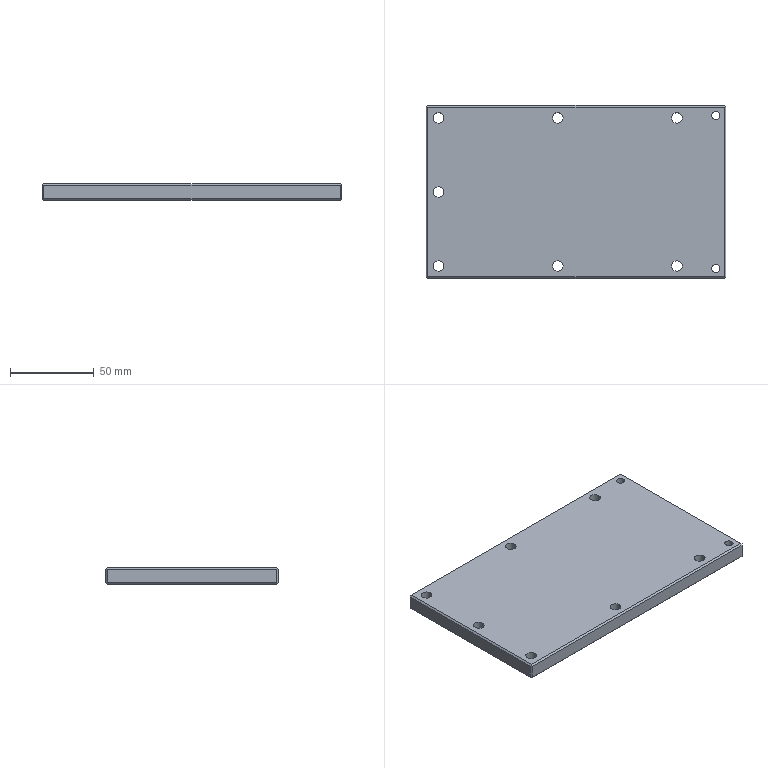Part | Creo | features DATUM PLANE 3, CHAMFER 1, COORDINATE SYSTEM 1, CURVE 1, PROTRUSION 1 | 1 solid | 36 faces | box 179.25 x 103.5 x 10 mm | volume 182337 mm3 | plane 18 | cylinder 18 | commonest cylinder face diameters 6.375 x14 4.875 x4
STEP:
#1=CARTESIAN_POINT('',(0.,0.,0.));
#2=DIRECTION('',(0.,0.,1.));
#3=DIRECTION('',(1.,0.,0.));
#4=AXIS2_PLACEMENT_3D('',#1,#2,#3);
#5=CARTESIAN_POINT('',(-88.63,50.75,0.));
#6=VERTEX_POINT('',#5);
#7=CARTESIAN_POINT('',(88.62,50.75,0.));
#8=VERTEX_POINT('',#7);
#9=CARTESIAN_POINT('',(-88.63,50.75,0.));
#10=DIRECTION('',(1.,0.,0.));
#11=VECTOR('',#10,177.25);
#12=LINE('',#9,#11);
#13=EDGE_CURVE('',#6,#8,#12,.T.);
#14=ORIENTED_EDGE('',*,*,#13,.F.);
#15=CARTESIAN_POINT('',(-88.63,-50.75,0.));
#16=VERTEX_POINT('',#15);
#17=CARTESIAN_POINT('',(-88.63,-50.75,0.));
#18=DIRECTION('',(0.,1.,0.));
#19=VECTOR('',#18,101.5);
#20=LINE('',#17,#19);
#21=EDGE_CURVE('',#16,#6,#20,.T.);
#22=ORIENTED_EDGE('',*,*,#21,.F.);
#23=CARTESIAN_POINT('',(88.62,-50.75,0.));
#24=VERTEX_POINT('',#23);
#25=CARTESIAN_POINT('',(88.62,-50.75,0.));
#26=DIRECTION('',(-1.,0.,0.));
#27=VECTOR('',#26,177.25);
#28=LINE('',#25,#27);
#29=EDGE_CURVE('',#24,#16,#28,.T.);
#30=ORIENTED_EDGE('',*,*,#29,.F.);
#31=CARTESIAN_POINT('',(88.62,50.75,0.));
#32=DIRECTION('',(0.,-1.,0.));
#33=VECTOR('',#32,101.5);
#34=LINE('',#31,#33);
#35=EDGE_CURVE('',#8,#24,#34,.T.);
#36=ORIENTED_EDGE('',*,*,#35,.F.);
#37=EDGE_LOOP('',(#14,#22,#30,#36));
#38=FACE_OUTER_BOUND('',#37,.F.);
#39=CARTESIAN_POINT('',(-78.942,-44.25,0.));
#40=VERTEX_POINT('',#39);
#41=CARTESIAN_POINT('',(-85.317,-44.25,0.));
#42=VERTEX_POINT('',#41);
#43=CARTESIAN_POINT('',(-82.13,-44.25,0.));
#44=DIRECTION('',(0.,0.,-1.));
#45=DIRECTION('',(1.,0.,0.));
#46=AXIS2_PLACEMENT_3D('',#43,#44,#45);
#47=CIRCLE('',#46,3.188);
#48=EDGE_CURVE('',#40,#42,#47,.T.);
#49=ORIENTED_EDGE('',*,*,#48,.T.);
#50=CARTESIAN_POINT('',(-82.13,-44.25,0.));
#51=DIRECTION('',(0.,0.,-1.));
#52=DIRECTION('',(-1.,0.,0.));
#53=AXIS2_PLACEMENT_3D('',#50,#51,#52);
#54=CIRCLE('',#53,3.188);
#55=EDGE_CURVE('',#42,#40,#54,.T.);
#56=ORIENTED_EDGE('',*,*,#55,.T.);
#57=EDGE_LOOP('',(#49,#56));
#58=FACE_BOUND('',#57,.F.);
#59=CARTESIAN_POINT('',(63.557,44.25,0.));
#60=VERTEX_POINT('',#59);
#61=CARTESIAN_POINT('',(57.182,44.25,0.));
#62=VERTEX_POINT('',#61);
#63=CARTESIAN_POINT('',(60.37,44.25,0.));
#64=DIRECTION('',(0.,0.,-1.));
#65=DIRECTION('',(1.,0.,0.));
#66=AXIS2_PLACEMENT_3D('',#63,#64,#65);
#67=CIRCLE('',#66,3.188);
#68=EDGE_CURVE('',#60,#62,#67,.T.);
#69=ORIENTED_EDGE('',*,*,#68,.T.);
#70=CARTESIAN_POINT('',(60.37,44.25,0.));
#71=DIRECTION('',(0.,0.,-1.));
#72=DIRECTION('',(-1.,0.,0.));
#73=AXIS2_PLACEMENT_3D('',#70,#71,#72);
#74=CIRCLE('',#73,3.188);
#75=EDGE_CURVE('',#62,#60,#74,.T.);
#76=ORIENTED_EDGE('',*,*,#75,.T.);
#77=EDGE_LOOP('',(#69,#76));
#78=FACE_BOUND('',#77,.F.);
#79=CARTESIAN_POINT('',(63.557,-44.25,0.));
#80=VERTEX_POINT('',#79);
#81=CARTESIAN_POINT('',(57.182,-44.25,0.));
#82=VERTEX_POINT('',#81);
#83=CARTESIAN_POINT('',(60.37,-44.25,0.));
#84=DIRECTION('',(0.,0.,-1.));
#85=DIRECTION('',(1.,0.,0.));
#86=AXIS2_PLACEMENT_3D('',#83,#84,#85);
#87=CIRCLE('',#86,3.188);
#88=EDGE_CURVE('',#80,#82,#87,.T.);
#89=ORIENTED_EDGE('',*,*,#88,.T.);
#90=CARTESIAN_POINT('',(60.37,-44.25,0.));
#91=DIRECTION('',(0.,0.,-1.));
#92=DIRECTION('',(-1.,0.,0.));
#93=AXIS2_PLACEMENT_3D('',#90,#91,#92);
#94=CIRCLE('',#93,3.188);
#95=EDGE_CURVE('',#82,#80,#94,.T.);
#96=ORIENTED_EDGE('',*,*,#95,.T.);
#97=EDGE_LOOP('',(#89,#96));
#98=FACE_BOUND('',#97,.F.);
#99=CARTESIAN_POINT('',(-7.692,44.25,0.));
#100=VERTEX_POINT('',#99);
#101=CARTESIAN_POINT('',(-14.068,44.25,0.));
#102=VERTEX_POINT('',#101);
#103=CARTESIAN_POINT('',(-10.88,44.25,0.));
#104=DIRECTION('',(0.,0.,-1.));
#105=DIRECTION('',(1.,0.,0.));
#106=AXIS2_PLACEMENT_3D('',#103,#104,#105);
#107=CIRCLE('',#106,3.188);
#108=EDGE_CURVE('',#100,#102,#107,.T.);
#109=ORIENTED_EDGE('',*,*,#108,.T.);
#110=CARTESIAN_POINT('',(-10.88,44.25,0.));
#111=DIRECTION('',(0.,0.,-1.));
#112=DIRECTION('',(-1.,0.,0.));
#113=AXIS2_PLACEMENT_3D('',#110,#111,#112);
#114=CIRCLE('',#113,3.188);
#115=EDGE_CURVE('',#102,#100,#114,.T.);
#116=ORIENTED_EDGE('',*,*,#115,.T.);
#117=EDGE_LOOP('',(#109,#116));
#118=FACE_BOUND('',#117,.F.);
#119=CARTESIAN_POINT('',(-7.692,-44.25,0.));
#120=VERTEX_POINT('',#119);
#121=CARTESIAN_POINT('',(-14.068,-44.25,0.));
#122=VERTEX_POINT('',#121);
#123=CARTESIAN_POINT('',(-10.88,-44.25,0.));
#124=DIRECTION('',(0.,0.,-1.));
#125=DIRECTION('',(1.,0.,0.));
#126=AXIS2_PLACEMENT_3D('',#123,#124,#125);
#127=CIRCLE('',#126,3.188);
#128=EDGE_CURVE('',#120,#122,#127,.T.);
#129=ORIENTED_EDGE('',*,*,#128,.T.);
#130=CARTESIAN_POINT('',(-10.88,-44.25,0.));
#131=DIRECTION('',(0.,0.,-1.));
#132=DIRECTION('',(-1.,0.,0.));
#133=AXIS2_PLACEMENT_3D('',#130,#131,#132);
#134=CIRCLE('',#133,3.188);
#135=EDGE_CURVE('',#122,#120,#134,.T.);
#136=ORIENTED_EDGE('',*,*,#135,.T.);
#137=EDGE_LOOP('',(#129,#136));
#138=FACE_BOUND('',#137,.F.);
#139=CARTESIAN_POINT('',(-78.942,0.,0.));
#140=VERTEX_POINT('',#139);
#141=CARTESIAN_POINT('',(-85.317,0.,0.));
#142=VERTEX_POINT('',#141);
#143=CARTESIAN_POINT('',(-82.13,0.,0.));
#144=DIRECTION('',(0.,0.,-1.));
#145=DIRECTION('',(1.,0.,0.));
#146=AXIS2_PLACEMENT_3D('',#143,#144,#145);
#147=CIRCLE('',#146,3.188);
#148=EDGE_CURVE('',#140,#142,#147,.T.);
#149=ORIENTED_EDGE('',*,*,#148,.T.);
#150=CARTESIAN_POINT('',(-82.13,0.,0.));
#151=DIRECTION('',(0.,0.,-1.));
#152=DIRECTION('',(-1.,0.,0.));
#153=AXIS2_PLACEMENT_3D('',#150,#151,#152);
#154=CIRCLE('',#153,3.188);
#155=EDGE_CURVE('',#142,#140,#154,.T.);
#156=ORIENTED_EDGE('',*,*,#155,.T.);
#157=EDGE_LOOP('',(#149,#156));
#158=FACE_BOUND('',#157,.F.);
#159=CARTESIAN_POINT('',(86.058,45.75,0.));
#160=VERTEX_POINT('',#159);
#161=CARTESIAN_POINT('',(81.183,45.75,0.));
#162=VERTEX_POINT('',#161);
#163=CARTESIAN_POINT('',(83.62,45.75,0.));
#164=DIRECTION('',(0.,0.,-1.));
#165=DIRECTION('',(1.,0.,0.));
#166=AXIS2_PLACEMENT_3D('',#163,#164,#165);
#167=CIRCLE('',#166,2.438);
#168=EDGE_CURVE('',#160,#162,#167,.T.);
#169=ORIENTED_EDGE('',*,*,#168,.T.);
#170=CARTESIAN_POINT('',(83.62,45.75,0.));
#171=DIRECTION('',(0.,0.,-1.));
#172=DIRECTION('',(-1.,0.,0.));
#173=AXIS2_PLACEMENT_3D('',#170,#171,#172);
#174=CIRCLE('',#173,2.438);
#175=EDGE_CURVE('',#162,#160,#174,.T.);
#176=ORIENTED_EDGE('',*,*,#175,.T.);
#177=EDGE_LOOP('',(#169,#176));
#178=FACE_BOUND('',#177,.F.);
#179=CARTESIAN_POINT('',(86.058,-45.75,0.));
#180=VERTEX_POINT('',#179);
#181=CARTESIAN_POINT('',(81.183,-45.75,0.));
#182=VERTEX_POINT('',#181);
#183=CARTESIAN_POINT('',(83.62,-45.75,0.));
#184=DIRECTION('',(0.,0.,-1.));
#185=DIRECTION('',(1.,0.,0.));
#186=AXIS2_PLACEMENT_3D('',#183,#184,#185);
#187=CIRCLE('',#186,2.438);
#188=EDGE_CURVE('',#180,#182,#187,.T.);
#189=ORIENTED_EDGE('',*,*,#188,.T.);
#190=CARTESIAN_POINT('',(83.62,-45.75,0.));
#191=DIRECTION('',(0.,0.,-1.));
#192=DIRECTION('',(-1.,0.,0.));
#193=AXIS2_PLACEMENT_3D('',#190,#191,#192);
#194=CIRCLE('',#193,2.438);
#195=EDGE_CURVE('',#182,#180,#194,.T.);
#196=ORIENTED_EDGE('',*,*,#195,.T.);
#197=EDGE_LOOP('',(#189,#196));
#198=FACE_BOUND('',#197,.F.);
#199=CARTESIAN_POINT('',(-78.942,44.25,0.));
#200=VERTEX_POINT('',#199);
#201=CARTESIAN_POINT('',(-85.317,44.25,0.));
#202=VERTEX_POINT('',#201);
#203=CARTESIAN_POINT('',(-82.13,44.25,0.));
#204=DIRECTION('',(0.,0.,-1.));
#205=DIRECTION('',(1.,0.,0.));
#206=AXIS2_PLACEMENT_3D('',#203,#204,#205);
#207=CIRCLE('',#206,3.188);
#208=EDGE_CURVE('',#200,#202,#207,.T.);
#209=ORIENTED_EDGE('',*,*,#208,.T.);
#210=CARTESIAN_POINT('',(-82.13,44.25,0.));
#211=DIRECTION('',(0.,0.,-1.));
#212=DIRECTION('',(-1.,0.,0.));
#213=AXIS2_PLACEMENT_3D('',#210,#211,#212);
#214=CIRCLE('',#213,3.188);
#215=EDGE_CURVE('',#202,#200,#214,.T.);
#216=ORIENTED_EDGE('',*,*,#215,.T.);
#217=EDGE_LOOP('',(#209,#216));
#218=FACE_BOUND('',#217,.F.);
#219=CARTESIAN_POINT('',(0.,0.,0.));
#220=DIRECTION('',(0.,0.,1.));
#221=DIRECTION('',(1.,0.,0.));
#222=AXIS2_PLACEMENT_3D('',#219,#220,#221);
#223=PLANE('',#222);
#224=ADVANCED_FACE('',(#38,#58,#78,#98,#118,#138,#158,#178,#198,#218),#223,.F.);
#225=ORIENTED_EDGE('',*,*,#208,.F.);
#226=CARTESIAN_POINT('',(-78.942,44.25,10.));
#227=VERTEX_POINT('',#226);
#228=CARTESIAN_POINT('',(-78.942,44.25,0.));
#229=DIRECTION('',(0.,0.,1.));
#230=VECTOR('',#229,10.);
#231=LINE('',#228,#230);
#232=EDGE_CURVE('',#200,#227,#231,.T.);
#233=ORIENTED_EDGE('',*,*,#232,.T.);
#234=CARTESIAN_POINT('',(-85.317,44.25,10.));
#235=VERTEX_POINT('',#234);
#236=CARTESIAN_POINT('',(-82.13,44.25,10.));
#237=DIRECTION('',(0.,0.,-1.));
#238=DIRECTION('',(1.,0.,0.));
#239=AXIS2_PLACEMENT_3D('',#236,#237,#238);
#240=CIRCLE('',#239,3.188);
#241=EDGE_CURVE('',#227,#235,#240,.T.);
#242=ORIENTED_EDGE('',*,*,#241,.T.);
#243=CARTESIAN_POINT('',(-85.317,44.25,0.));
#244=DIRECTION('',(0.,0.,1.));
#245=VECTOR('',#244,10.);
#246=LINE('',#243,#245);
#247=EDGE_CURVE('',#202,#235,#246,.T.);
#248=ORIENTED_EDGE('',*,*,#247,.F.);
#249=EDGE_LOOP('',(#225,#233,#242,#248));
#250=FACE_OUTER_BOUND('',#249,.F.);
#251=CARTESIAN_POINT('',(-82.13,44.25,0.));
#252=DIRECTION('',(0.,0.,1.));
#253=DIRECTION('',(1.,0.,0.));
#254=AXIS2_PLACEMENT_3D('',#251,#252,#253);
#255=CYLINDRICAL_SURFACE('',#254,3.188);
#256=ADVANCED_FACE('',(#250),#255,.F.);
#257=ORIENTED_EDGE('',*,*,#215,.F.);
#258=ORIENTED_EDGE('',*,*,#247,.T.);
#259=CARTESIAN_POINT('',(-82.13,44.25,10.));
#260=DIRECTION('',(0.,0.,-1.));
#261=DIRECTION('',(-1.,0.,0.));
#262=AXIS2_PLACEMENT_3D('',#259,#260,#261);
#263=CIRCLE('',#262,3.188);
#264=EDGE_CURVE('',#235,#227,#263,.T.);
#265=ORIENTED_EDGE('',*,*,#264,.T.);
#266=ORIENTED_EDGE('',*,*,#232,.F.);
#267=EDGE_LOOP('',(#257,#258,#265,#266));
#268=FACE_OUTER_BOUND('',#267,.F.);
#269=CARTESIAN_POINT('',(-82.13,44.25,0.));
#270=DIRECTION('',(0.,0.,1.));
#271=DIRECTION('',(1.,0.,0.));
#272=AXIS2_PLACEMENT_3D('',#269,#270,#271);
#273=CYLINDRICAL_SURFACE('',#272,3.188);
#274=ADVANCED_FACE('',(#268),#273,.F.);
#275=CARTESIAN_POINT('',(88.62,-50.75,10.));
#276=VERTEX_POINT('',#275);
#277=CARTESIAN_POINT('',(88.62,50.75,10.));
#278=VERTEX_POINT('',#277);
#279=CARTESIAN_POINT('',(88.62,-50.75,10.));
#280=DIRECTION('',(0.,1.,0.));
#281=VECTOR('',#280,101.5);
#282=LINE('',#279,#281);
#283=EDGE_CURVE('',#276,#278,#282,.T.);
#284=ORIENTED_EDGE('',*,*,#283,.F.);
#285=CARTESIAN_POINT('',(-88.63,-50.75,10.));
#286=VERTEX_POINT('',#285);
#287=CARTESIAN_POINT('',(-88.63,-50.75,10.));
#288=DIRECTION('',(1.,0.,0.));
#289=VECTOR('',#288,177.25);
#290=LINE('',#287,#289);
#291=EDGE_CURVE('',#286,#276,#290,.T.);
#292=ORIENTED_EDGE('',*,*,#291,.F.);
#293=CARTESIAN_POINT('',(-88.63,50.75,10.));
#294=VERTEX_POINT('',#293);
#295=CARTESIAN_POINT('',(-88.63,50.75,10.));
#296=DIRECTION('',(0.,-1.,0.));
#297=VECTOR('',#296,101.5);
#298=LINE('',#295,#297);
#299=EDGE_CURVE('',#294,#286,#298,.T.);
#300=ORIENTED_EDGE('',*,*,#299,.F.);
#301=CARTESIAN_POINT('',(88.62,50.75,10.));
#302=DIRECTION('',(-1.,0.,0.));
#303=VECTOR('',#302,177.25);
#304=LINE('',#301,#303);
#305=EDGE_CURVE('',#278,#294,#304,.T.);
#306=ORIENTED_EDGE('',*,*,#305,.F.);
#307=EDGE_LOOP('',(#284,#292,#300,#306));
#308=FACE_OUTER_BOUND('',#307,.F.);
#309=CARTESIAN_POINT('',(-78.942,-44.25,10.));
#310=VERTEX_POINT('',#309);
#311=CARTESIAN_POINT('',(-85.317,-44.25,10.));
#312=VERTEX_POINT('',#311);
#313=CARTESIAN_POINT('',(-82.13,-44.25,10.));
#314=DIRECTION('',(0.,0.,-1.));
#315=DIRECTION('',(1.,0.,0.));
#316=AXIS2_PLACEMENT_3D('',#313,#314,#315);
#317=CIRCLE('',#316,3.188);
#318=EDGE_CURVE('',#310,#312,#317,.T.);
#319=ORIENTED_EDGE('',*,*,#318,.F.);
#320=CARTESIAN_POINT('',(-82.13,-44.25,10.));
#321=DIRECTION('',(0.,0.,-1.));
#322=DIRECTION('',(-1.,0.,0.));
#323=AXIS2_PLACEMENT_3D('',#320,#321,#322);
#324=CIRCLE('',#323,3.188);
#325=EDGE_CURVE('',#312,#310,#324,.T.);
#326=ORIENTED_EDGE('',*,*,#325,.F.);
#327=EDGE_LOOP('',(#319,#326));
#328=FACE_BOUND('',#327,.F.);
#329=CARTESIAN_POINT('',(63.557,44.25,10.));
#330=VERTEX_POINT('',#329);
#331=CARTESIAN_POINT('',(57.182,44.25,10.));
#332=VERTEX_POINT('',#331);
#333=CARTESIAN_POINT('',(60.37,44.25,10.));
#334=DIRECTION('',(0.,0.,-1.));
#335=DIRECTION('',(1.,0.,0.));
#336=AXIS2_PLACEMENT_3D('',#333,#334,#335);
#337=CIRCLE('',#336,3.188);
#338=EDGE_CURVE('',#330,#332,#337,.T.);
#339=ORIENTED_EDGE('',*,*,#338,.F.);
#340=CARTESIAN_POINT('',(60.37,44.25,10.));
#341=DIRECTION('',(0.,0.,-1.));
#342=DIRECTION('',(-1.,0.,0.));
#343=AXIS2_PLACEMENT_3D('',#340,#341,#342);
#344=CIRCLE('',#343,3.188);
#345=EDGE_CURVE('',#332,#330,#344,.T.);
#346=ORIENTED_EDGE('',*,*,#345,.F.);
#347=EDGE_LOOP('',(#339,#346));
#348=FACE_BOUND('',#347,.F.);
#349=CARTESIAN_POINT('',(63.557,-44.25,10.));
#350=VERTEX_POINT('',#349);
#351=CARTESIAN_POINT('',(57.182,-44.25,10.));
#352=VERTEX_POINT('',#351);
#353=CARTESIAN_POINT('',(60.37,-44.25,10.));
#354=DIRECTION('',(0.,0.,-1.));
#355=DIRECTION('',(1.,0.,0.));
#356=AXIS2_PLACEMENT_3D('',#353,#354,#355);
#357=CIRCLE('',#356,3.188);
#358=EDGE_CURVE('',#350,#352,#357,.T.);
#359=ORIENTED_EDGE('',*,*,#358,.F.);
#360=CARTESIAN_POINT('',(60.37,-44.25,10.));
#361=DIRECTION('',(0.,0.,-1.));
#362=DIRECTION('',(-1.,0.,0.));
#363=AXIS2_PLACEMENT_3D('',#360,#361,#362);
#364=CIRCLE('',#363,3.188);
#365=EDGE_CURVE('',#352,#350,#364,.T.);
#366=ORIENTED_EDGE('',*,*,#365,.F.);
#367=EDGE_LOOP('',(#359,#366));
#368=FACE_BOUND('',#367,.F.);
#369=CARTESIAN_POINT('',(-7.692,44.25,10.));
#370=VERTEX_POINT('',#369);
#371=CARTESIAN_POINT('',(-14.068,44.25,10.));
#372=VERTEX_POINT('',#371);
#373=CARTESIAN_POINT('',(-10.88,44.25,10.));
#374=DIRECTION('',(0.,0.,-1.));
#375=DIRECTION('',(1.,0.,0.));
#376=AXIS2_PLACEMENT_3D('',#373,#374,#375);
#377=CIRCLE('',#376,3.188);
#378=EDGE_CURVE('',#370,#372,#377,.T.);
#379=ORIENTED_EDGE('',*,*,#378,.F.);
#380=CARTESIAN_POINT('',(-10.88,44.25,10.));
#381=DIRECTION('',(0.,0.,-1.));
#382=DIRECTION('',(-1.,0.,0.));
#383=AXIS2_PLACEMENT_3D('',#380,#381,#382);
#384=CIRCLE('',#383,3.188);
#385=EDGE_CURVE('',#372,#370,#384,.T.);
#386=ORIENTED_EDGE('',*,*,#385,.F.);
#387=EDGE_LOOP('',(#379,#386));
#388=FACE_BOUND('',#387,.F.);
#389=CARTESIAN_POINT('',(-7.692,-44.25,10.));
#390=VERTEX_POINT('',#389);
#391=CARTESIAN_POINT('',(-14.068,-44.25,10.));
#392=VERTEX_POINT('',#391);
#393=CARTESIAN_POINT('',(-10.88,-44.25,10.));
#394=DIRECTION('',(0.,0.,-1.));
#395=DIRECTION('',(1.,0.,0.));
#396=AXIS2_PLACEMENT_3D('',#393,#394,#395);
#397=CIRCLE('',#396,3.188);
#398=EDGE_CURVE('',#390,#392,#397,.T.);
#399=ORIENTED_EDGE('',*,*,#398,.F.);
#400=CARTESIAN_POINT('',(-10.88,-44.25,10.));
#401=DIRECTION('',(0.,0.,-1.));
#402=DIRECTION('',(-1.,0.,0.));
#403=AXIS2_PLACEMENT_3D('',#400,#401,#402);
#404=CIRCLE('',#403,3.188);
#405=EDGE_CURVE('',#392,#390,#404,.T.);
#406=ORIENTED_EDGE('',*,*,#405,.F.);
#407=EDGE_LOOP('',(#399,#406));
#408=FACE_BOUND('',#407,.F.);
#409=CARTESIAN_POINT('',(-78.942,0.,10.));
#410=VERTEX_POINT('',#409);
#411=CARTESIAN_POINT('',(-85.317,0.,10.));
#412=VERTEX_POINT('',#411);
#413=CARTESIAN_POINT('',(-82.13,0.,10.));
#414=DIRECTION('',(0.,0.,-1.));
#415=DIRECTION('',(1.,0.,0.));
#416=AXIS2_PLACEMENT_3D('',#413,#414,#415);
#417=CIRCLE('',#416,3.188);
#418=EDGE_CURVE('',#410,#412,#417,.T.);
#419=ORIENTED_EDGE('',*,*,#418,.F.);
#420=CARTESIAN_POINT('',(-82.13,0.,10.));
#421=DIRECTION('',(0.,0.,-1.));
#422=DIRECTION('',(-1.,0.,0.));
#423=AXIS2_PLACEMENT_3D('',#420,#421,#422);
#424=CIRCLE('',#423,3.188);
#425=EDGE_CURVE('',#412,#410,#424,.T.);
#426=ORIENTED_EDGE('',*,*,#425,.F.);
#427=EDGE_LOOP('',(#419,#426));
#428=FACE_BOUND('',#427,.F.);
#429=CARTESIAN_POINT('',(86.058,45.75,10.));
#430=VERTEX_POINT('',#429);
#431=CARTESIAN_POINT('',(81.183,45.75,10.));
#432=VERTEX_POINT('',#431);
#433=CARTESIAN_POINT('',(83.62,45.75,10.));
#434=DIRECTION('',(0.,0.,-1.));
#435=DIRECTION('',(1.,0.,0.));
#436=AXIS2_PLACEMENT_3D('',#433,#434,#435);
#437=CIRCLE('',#436,2.438);
#438=EDGE_CURVE('',#430,#432,#437,.T.);
#439=ORIENTED_EDGE('',*,*,#438,.F.);
#440=CARTESIAN_POINT('',(83.62,45.75,10.));
#441=DIRECTION('',(0.,0.,-1.));
#442=DIRECTION('',(-1.,0.,0.));
#443=AXIS2_PLACEMENT_3D('',#440,#441,#442);
#444=CIRCLE('',#443,2.438);
#445=EDGE_CURVE('',#432,#430,#444,.T.);
#446=ORIENTED_EDGE('',*,*,#445,.F.);
#447=EDGE_LOOP('',(#439,#446));
#448=FACE_BOUND('',#447,.F.);
#449=CARTESIAN_POINT('',(86.058,-45.75,10.));
#450=VERTEX_POINT('',#449);
#451=CARTESIAN_POINT('',(81.183,-45.75,10.));
#452=VERTEX_POINT('',#451);
#453=CARTESIAN_POINT('',(83.62,-45.75,10.));
#454=DIRECTION('',(0.,0.,-1.));
#455=DIRECTION('',(1.,0.,0.));
#456=AXIS2_PLACEMENT_3D('',#453,#454,#455);
#457=CIRCLE('',#456,2.438);
#458=EDGE_CURVE('',#450,#452,#457,.T.);
#459=ORIENTED_EDGE('',*,*,#458,.F.);
#460=CARTESIAN_POINT('',(83.62,-45.75,10.));
#461=DIRECTION('',(0.,0.,-1.));
#462=DIRECTION('',(-1.,0.,0.));
#463=AXIS2_PLACEMENT_3D('',#460,#461,#462);
#464=CIRCLE('',#463,2.438);
#465=EDGE_CURVE('',#452,#450,#464,.T.);
#466=ORIENTED_EDGE('',*,*,#465,.F.);
#467=EDGE_LOOP('',(#459,#466));
#468=FACE_BOUND('',#467,.F.);
#469=ORIENTED_EDGE('',*,*,#241,.F.);
#470=ORIENTED_EDGE('',*,*,#264,.F.);
#471=EDGE_LOOP('',(#469,#470));
#472=FACE_BOUND('',#471,.F.);
#473=CARTESIAN_POINT('',(0.,0.,10.));
#474=DIRECTION('',(0.,0.,1.));
#475=DIRECTION('',(1.,0.,0.));
#476=AXIS2_PLACEMENT_3D('',#473,#474,#475);
#477=PLANE('',#476);
#478=ADVANCED_FACE('',(#308,#328,#348,#368,#388,#408,#428,#448,#468,#472),#477,.T.);
#479=ORIENTED_EDGE('',*,*,#48,.F.);
#480=CARTESIAN_POINT('',(-78.942,-44.25,0.));
#481=DIRECTION('',(0.,0.,1.));
#482=VECTOR('',#481,10.);
#483=LINE('',#480,#482);
#484=EDGE_CURVE('',#40,#310,#483,.T.);
#485=ORIENTED_EDGE('',*,*,#484,.T.);
#486=ORIENTED_EDGE('',*,*,#318,.T.);
#487=CARTESIAN_POINT('',(-85.317,-44.25,0.));
#488=DIRECTION('',(0.,0.,1.));
#489=VECTOR('',#488,10.);
#490=LINE('',#487,#489);
#491=EDGE_CURVE('',#42,#312,#490,.T.);
#492=ORIENTED_EDGE('',*,*,#491,.F.);
#493=EDGE_LOOP('',(#479,#485,#486,#492));
#494=FACE_OUTER_BOUND('',#493,.F.);
#495=CARTESIAN_POINT('',(-82.13,-44.25,0.));
#496=DIRECTION('',(0.,0.,1.));
#497=DIRECTION('',(1.,0.,0.));
#498=AXIS2_PLACEMENT_3D('',#495,#496,#497);
#499=CYLINDRICAL_SURFACE('',#498,3.188);
#500=ADVANCED_FACE('',(#494),#499,.F.);
#501=ORIENTED_EDGE('',*,*,#55,.F.);
#502=ORIENTED_EDGE('',*,*,#491,.T.);
#503=ORIENTED_EDGE('',*,*,#325,.T.);
#504=ORIENTED_EDGE('',*,*,#484,.F.);
#505=EDGE_LOOP('',(#501,#502,#503,#504));
#506=FACE_OUTER_BOUND('',#505,.F.);
#507=CARTESIAN_POINT('',(-82.13,-44.25,0.));
#508=DIRECTION('',(0.,0.,1.));
#509=DIRECTION('',(1.,0.,0.));
#510=AXIS2_PLACEMENT_3D('',#507,#508,#509);
#511=CYLINDRICAL_SURFACE('',#510,3.188);
#512=ADVANCED_FACE('',(#506),#511,.F.);
#513=ORIENTED_EDGE('',*,*,#68,.F.);
#514=CARTESIAN_POINT('',(63.557,44.25,0.));
#515=DIRECTION('',(0.,0.,1.));
#516=VECTOR('',#515,10.);
#517=LINE('',#514,#516);
#518=EDGE_CURVE('',#60,#330,#517,.T.);
#519=ORIENTED_EDGE('',*,*,#518,.T.);
#520=ORIENTED_EDGE('',*,*,#338,.T.);
#521=CARTESIAN_POINT('',(57.182,44.25,0.));
#522=DIRECTION('',(0.,0.,1.));
#523=VECTOR('',#522,10.);
#524=LINE('',#521,#523);
#525=EDGE_CURVE('',#62,#332,#524,.T.);
#526=ORIENTED_EDGE('',*,*,#525,.F.);
#527=EDGE_LOOP('',(#513,#519,#520,#526));
#528=FACE_OUTER_BOUND('',#527,.F.);
#529=CARTESIAN_POINT('',(60.37,44.25,0.));
#530=DIRECTION('',(0.,0.,1.));
#531=DIRECTION('',(1.,0.,0.));
#532=AXIS2_PLACEMENT_3D('',#529,#530,#531);
#533=CYLINDRICAL_SURFACE('',#532,3.188);
#534=ADVANCED_FACE('',(#528),#533,.F.);
#535=ORIENTED_EDGE('',*,*,#75,.F.);
#536=ORIENTED_EDGE('',*,*,#525,.T.);
#537=ORIENTED_EDGE('',*,*,#345,.T.);
#538=ORIENTED_EDGE('',*,*,#518,.F.);
#539=EDGE_LOOP('',(#535,#536,#537,#538));
#540=FACE_OUTER_BOUND('',#539,.F.);
#541=CARTESIAN_POINT('',(60.37,44.25,0.));
#542=DIRECTION('',(0.,0.,1.));
#543=DIRECTION('',(1.,0.,0.));
#544=AXIS2_PLACEMENT_3D('',#541,#542,#543);
#545=CYLINDRICAL_SURFACE('',#544,3.188);
#546=ADVANCED_FACE('',(#540),#545,.F.);
#547=ORIENTED_EDGE('',*,*,#88,.F.);
#548=CARTESIAN_POINT('',(63.557,-44.25,0.));
#549=DIRECTION('',(0.,0.,1.));
#550=VECTOR('',#549,10.);
#551=LINE('',#548,#550);
#552=EDGE_CURVE('',#80,#350,#551,.T.);
#553=ORIENTED_EDGE('',*,*,#552,.T.);
#554=ORIENTED_EDGE('',*,*,#358,.T.);
#555=CARTESIAN_POINT('',(57.182,-44.25,0.));
#556=DIRECTION('',(0.,0.,1.));
#557=VECTOR('',#556,10.);
#558=LINE('',#555,#557);
#559=EDGE_CURVE('',#82,#352,#558,.T.);
#560=ORIENTED_EDGE('',*,*,#559,.F.);
#561=EDGE_LOOP('',(#547,#553,#554,#560));
#562=FACE_OUTER_BOUND('',#561,.F.);
#563=CARTESIAN_POINT('',(60.37,-44.25,0.));
#564=DIRECTION('',(0.,0.,1.));
#565=DIRECTION('',(1.,0.,0.));
#566=AXIS2_PLACEMENT_3D('',#563,#564,#565);
#567=CYLINDRICAL_SURFACE('',#566,3.188);
#568=ADVANCED_FACE('',(#562),#567,.F.);
#569=ORIENTED_EDGE('',*,*,#95,.F.);
#570=ORIENTED_EDGE('',*,*,#559,.T.);
#571=ORIENTED_EDGE('',*,*,#365,.T.);
#572=ORIENTED_EDGE('',*,*,#552,.F.);
#573=EDGE_LOOP('',(#569,#570,#571,#572));
#574=FACE_OUTER_BOUND('',#573,.F.);
#575=CARTESIAN_POINT('',(60.37,-44.25,0.));
#576=DIRECTION('',(0.,0.,1.));
#577=DIRECTION('',(1.,0.,0.));
#578=AXIS2_PLACEMENT_3D('',#575,#576,#577);
#579=CYLINDRICAL_SURFACE('',#578,3.188);
#580=ADVANCED_FACE('',(#574),#579,.F.);
#581=ORIENTED_EDGE('',*,*,#108,.F.);
#582=CARTESIAN_POINT('',(-7.692,44.25,0.));
#583=DIRECTION('',(0.,0.,1.));
#584=VECTOR('',#583,10.);
#585=LINE('',#582,#584);
#586=EDGE_CURVE('',#100,#370,#585,.T.);
#587=ORIENTED_EDGE('',*,*,#586,.T.);
#588=ORIENTED_EDGE('',*,*,#378,.T.);
#589=CARTESIAN_POINT('',(-14.068,44.25,0.));
#590=DIRECTION('',(0.,0.,1.));
#591=VECTOR('',#590,10.);
#592=LINE('',#589,#591);
#593=EDGE_CURVE('',#102,#372,#592,.T.);
#594=ORIENTED_EDGE('',*,*,#593,.F.);
#595=EDGE_LOOP('',(#581,#587,#588,#594));
#596=FACE_OUTER_BOUND('',#595,.F.);
#597=CARTESIAN_POINT('',(-10.88,44.25,0.));
#598=DIRECTION('',(0.,0.,1.));
#599=DIRECTION('',(1.,0.,0.));
#600=AXIS2_PLACEMENT_3D('',#597,#598,#599);
#601=CYLINDRICAL_SURFACE('',#600,3.188);
#602=ADVANCED_FACE('',(#596),#601,.F.);
#603=ORIENTED_EDGE('',*,*,#115,.F.);
#604=ORIENTED_EDGE('',*,*,#593,.T.);
#605=ORIENTED_EDGE('',*,*,#385,.T.);
#606=ORIENTED_EDGE('',*,*,#586,.F.);
#607=EDGE_LOOP('',(#603,#604,#605,#606));
#608=FACE_OUTER_BOUND('',#607,.F.);
#609=CARTESIAN_POINT('',(-10.88,44.25,0.));
#610=DIRECTION('',(0.,0.,1.));
#611=DIRECTION('',(1.,0.,0.));
#612=AXIS2_PLACEMENT_3D('',#609,#610,#611);
#613=CYLINDRICAL_SURFACE('',#612,3.188);
#614=ADVANCED_FACE('',(#608),#613,.F.);
#615=ORIENTED_EDGE('',*,*,#128,.F.);
#616=CARTESIAN_POINT('',(-7.692,-44.25,0.));
#617=DIRECTION('',(0.,0.,1.));
#618=VECTOR('',#617,10.);
#619=LINE('',#616,#618);
#620=EDGE_CURVE('',#120,#390,#619,.T.);
#621=ORIENTED_EDGE('',*,*,#620,.T.);
#622=ORIENTED_EDGE('',*,*,#398,.T.);
#623=CARTESIAN_POINT('',(-14.068,-44.25,0.));
#624=DIRECTION('',(0.,0.,1.));
#625=VECTOR('',#624,10.);
#626=LINE('',#623,#625);
#627=EDGE_CURVE('',#122,#392,#626,.T.);
#628=ORIENTED_EDGE('',*,*,#627,.F.);
#629=EDGE_LOOP('',(#615,#621,#622,#628));
#630=FACE_OUTER_BOUND('',#629,.F.);
#631=CARTESIAN_POINT('',(-10.88,-44.25,0.));
#632=DIRECTION('',(0.,0.,1.));
#633=DIRECTION('',(1.,0.,0.));
#634=AXIS2_PLACEMENT_3D('',#631,#632,#633);
#635=CYLINDRICAL_SURFACE('',#634,3.188);
#636=ADVANCED_FACE('',(#630),#635,.F.);
#637=ORIENTED_EDGE('',*,*,#135,.F.);
#638=ORIENTED_EDGE('',*,*,#627,.T.);
#639=ORIENTED_EDGE('',*,*,#405,.T.);
#640=ORIENTED_EDGE('',*,*,#620,.F.);
#641=EDGE_LOOP('',(#637,#638,#639,#640));
#642=FACE_OUTER_BOUND('',#641,.F.);
#643=CARTESIAN_POINT('',(-10.88,-44.25,0.));
#644=DIRECTION('',(0.,0.,1.));
#645=DIRECTION('',(1.,0.,0.));
#646=AXIS2_PLACEMENT_3D('',#643,#644,#645);
#647=CYLINDRICAL_SURFACE('',#646,3.188);
#648=ADVANCED_FACE('',(#642),#647,.F.);
#649=ORIENTED_EDGE('',*,*,#148,.F.);
#650=CARTESIAN_POINT('',(-78.942,0.,0.));
#651=DIRECTION('',(0.,0.,1.));
#652=VECTOR('',#651,10.);
#653=LINE('',#650,#652);
#654=EDGE_CURVE('',#140,#410,#653,.T.);
#655=ORIENTED_EDGE('',*,*,#654,.T.);
#656=ORIENTED_EDGE('',*,*,#418,.T.);
#657=CARTESIAN_POINT('',(-85.317,0.,0.));
#658=DIRECTION('',(0.,0.,1.));
#659=VECTOR('',#658,10.);
#660=LINE('',#657,#659);
#661=EDGE_CURVE('',#142,#412,#660,.T.);
#662=ORIENTED_EDGE('',*,*,#661,.F.);
#663=EDGE_LOOP('',(#649,#655,#656,#662));
#664=FACE_OUTER_BOUND('',#663,.F.);
#665=CARTESIAN_POINT('',(-82.13,0.,0.));
#666=DIRECTION('',(0.,0.,1.));
#667=DIRECTION('',(1.,0.,0.));
#668=AXIS2_PLACEMENT_3D('',#665,#666,#667);
#669=CYLINDRICAL_SURFACE('',#668,3.188);
#670=ADVANCED_FACE('',(#664),#669,.F.);
#671=ORIENTED_EDGE('',*,*,#155,.F.);
#672=ORIENTED_EDGE('',*,*,#661,.T.);
#673=ORIENTED_EDGE('',*,*,#425,.T.);
#674=ORIENTED_EDGE('',*,*,#654,.F.);
#675=EDGE_LOOP('',(#671,#672,#673,#674));
#676=FACE_OUTER_BOUND('',#675,.F.);
#677=CARTESIAN_POINT('',(-82.13,0.,0.));
#678=DIRECTION('',(0.,0.,1.));
#679=DIRECTION('',(1.,0.,0.));
#680=AXIS2_PLACEMENT_3D('',#677,#678,#679);
#681=CYLINDRICAL_SURFACE('',#680,3.188);
#682=ADVANCED_FACE('',(#676),#681,.F.);
#683=ORIENTED_EDGE('',*,*,#168,.F.);
#684=CARTESIAN_POINT('',(86.058,45.75,0.));
#685=DIRECTION('',(0.,0.,1.));
#686=VECTOR('',#685,10.);
#687=LINE('',#684,#686);
#688=EDGE_CURVE('',#160,#430,#687,.T.);
#689=ORIENTED_EDGE('',*,*,#688,.T.);
#690=ORIENTED_EDGE('',*,*,#438,.T.);
#691=CARTESIAN_POINT('',(81.183,45.75,0.));
#692=DIRECTION('',(0.,0.,1.));
#693=VECTOR('',#692,10.);
#694=LINE('',#691,#693);
#695=EDGE_CURVE('',#162,#432,#694,.T.);
#696=ORIENTED_EDGE('',*,*,#695,.F.);
#697=EDGE_LOOP('',(#683,#689,#690,#696));
#698=FACE_OUTER_BOUND('',#697,.F.);
#699=CARTESIAN_POINT('',(83.62,45.75,0.));
#700=DIRECTION('',(0.,0.,1.));
#701=DIRECTION('',(1.,0.,0.));
#702=AXIS2_PLACEMENT_3D('',#699,#700,#701);
#703=CYLINDRICAL_SURFACE('',#702,2.438);
#704=ADVANCED_FACE('',(#698),#703,.F.);
#705=ORIENTED_EDGE('',*,*,#175,.F.);
#706=ORIENTED_EDGE('',*,*,#695,.T.);
#707=ORIENTED_EDGE('',*,*,#445,.T.);
#708=ORIENTED_EDGE('',*,*,#688,.F.);
#709=EDGE_LOOP('',(#705,#706,#707,#708));
#710=FACE_OUTER_BOUND('',#709,.F.);
#711=CARTESIAN_POINT('',(83.62,45.75,0.));
#712=DIRECTION('',(0.,0.,1.));
#713=DIRECTION('',(1.,0.,0.));
#714=AXIS2_PLACEMENT_3D('',#711,#712,#713);
#715=CYLINDRICAL_SURFACE('',#714,2.438);
#716=ADVANCED_FACE('',(#710),#715,.F.);
#717=ORIENTED_EDGE('',*,*,#188,.F.);
#718=CARTESIAN_POINT('',(86.058,-45.75,0.));
#719=DIRECTION('',(0.,0.,1.));
#720=VECTOR('',#719,10.);
#721=LINE('',#718,#720);
#722=EDGE_CURVE('',#180,#450,#721,.T.);
#723=ORIENTED_EDGE('',*,*,#722,.T.);
#724=ORIENTED_EDGE('',*,*,#458,.T.);
#725=CARTESIAN_POINT('',(81.183,-45.75,0.));
#726=DIRECTION('',(0.,0.,1.));
#727=VECTOR('',#726,10.);
#728=LINE('',#725,#727);
#729=EDGE_CURVE('',#182,#452,#728,.T.);
#730=ORIENTED_EDGE('',*,*,#729,.F.);
#731=EDGE_LOOP('',(#717,#723,#724,#730));
#732=FACE_OUTER_BOUND('',#731,.F.);
#733=CARTESIAN_POINT('',(83.62,-45.75,0.));
#734=DIRECTION('',(0.,0.,1.));
#735=DIRECTION('',(1.,0.,0.));
#736=AXIS2_PLACEMENT_3D('',#733,#734,#735);
#737=CYLINDRICAL_SURFACE('',#736,2.438);
#738=ADVANCED_FACE('',(#732),#737,.F.);
#739=ORIENTED_EDGE('',*,*,#195,.F.);
#740=ORIENTED_EDGE('',*,*,#729,.T.);
#741=ORIENTED_EDGE('',*,*,#465,.T.);
#742=ORIENTED_EDGE('',*,*,#722,.F.);
#743=EDGE_LOOP('',(#739,#740,#741,#742));
#744=FACE_OUTER_BOUND('',#743,.F.);
#745=CARTESIAN_POINT('',(83.62,-45.75,0.));
#746=DIRECTION('',(0.,0.,1.));
#747=DIRECTION('',(1.,0.,0.));
#748=AXIS2_PLACEMENT_3D('',#745,#746,#747);
#749=CYLINDRICAL_SURFACE('',#748,2.438);
#750=ADVANCED_FACE('',(#744),#749,.F.);
#751=CARTESIAN_POINT('',(89.62,-50.75,9.));
#752=VERTEX_POINT('',#751);
#753=CARTESIAN_POINT('',(89.62,50.75,9.));
#754=VERTEX_POINT('',#753);
#755=CARTESIAN_POINT('',(89.62,-50.75,9.));
#756=DIRECTION('',(0.,1.,0.));
#757=VECTOR('',#756,101.5);
#758=LINE('',#755,#757);
#759=EDGE_CURVE('',#752,#754,#758,.T.);
#760=ORIENTED_EDGE('',*,*,#759,.F.);
#761=CARTESIAN_POINT('',(89.12,-51.25,9.5));
#762=VERTEX_POINT('',#761);
#763=CARTESIAN_POINT('',(89.62,-50.75,9.));
#764=DIRECTION('',(-0.5774,-0.5774,0.5774));
#765=VECTOR('',#764,0.866);
#766=LINE('',#763,#765);
#767=EDGE_CURVE('',#752,#762,#766,.T.);
#768=ORIENTED_EDGE('',*,*,#767,.T.);
#769=CARTESIAN_POINT('',(88.62,-50.75,10.));
#770=DIRECTION('',(0.5774,-0.5774,-0.5774));
#771=VECTOR('',#770,0.866);
#772=LINE('',#769,#771);
#773=EDGE_CURVE('',#276,#762,#772,.T.);
#774=ORIENTED_EDGE('',*,*,#773,.F.);
#775=ORIENTED_EDGE('',*,*,#283,.T.);
#776=CARTESIAN_POINT('',(89.12,51.25,9.5));
#777=VERTEX_POINT('',#776);
#778=CARTESIAN_POINT('',(88.62,50.75,10.));
#779=DIRECTION('',(0.5774,0.5774,-0.5774));
#780=VECTOR('',#779,0.866);
#781=LINE('',#778,#780);
#782=EDGE_CURVE('',#278,#777,#781,.T.);
#783=ORIENTED_EDGE('',*,*,#782,.T.);
#784=CARTESIAN_POINT('',(89.12,51.25,9.5));
#785=DIRECTION('',(0.5774,-0.5774,-0.5774));
#786=VECTOR('',#785,0.866);
#787=LINE('',#784,#786);
#788=EDGE_CURVE('',#777,#754,#787,.T.);
#789=ORIENTED_EDGE('',*,*,#788,.T.);
#790=EDGE_LOOP('',(#760,#768,#774,#775,#783,#789));
#791=FACE_OUTER_BOUND('',#790,.F.);
#792=CARTESIAN_POINT('',(89.12,0.,9.5));
#793=DIRECTION('',(0.7071,0.,0.7071));
#794=DIRECTION('',(0.7071,0.,-0.7071));
#795=AXIS2_PLACEMENT_3D('',#792,#793,#794);
#796=PLANE('',#795);
#797=ADVANCED_FACE('',(#791),#796,.T.);
#798=CARTESIAN_POINT('',(89.62,-50.75,1.));
#799=VERTEX_POINT('',#798);
#800=CARTESIAN_POINT('',(89.62,-50.75,9.));
#801=DIRECTION('',(0.,0.,-1.));
#802=VECTOR('',#801,8.);
#803=LINE('',#800,#802);
#804=EDGE_CURVE('',#752,#799,#803,.T.);
#805=ORIENTED_EDGE('',*,*,#804,.F.);
#806=ORIENTED_EDGE('',*,*,#759,.T.);
#807=CARTESIAN_POINT('',(89.62,50.75,1.));
#808=VERTEX_POINT('',#807);
#809=CARTESIAN_POINT('',(89.62,50.75,9.));
#810=DIRECTION('',(0.,0.,-1.));
#811=VECTOR('',#810,8.);
#812=LINE('',#809,#811);
#813=EDGE_CURVE('',#754,#808,#812,.T.);
#814=ORIENTED_EDGE('',*,*,#813,.T.);
#815=CARTESIAN_POINT('',(89.62,50.75,1.));
#816=DIRECTION('',(0.,-1.,0.));
#817=VECTOR('',#816,101.5);
#818=LINE('',#815,#817);
#819=EDGE_CURVE('',#808,#799,#818,.T.);
#820=ORIENTED_EDGE('',*,*,#819,.T.);
#821=EDGE_LOOP('',(#805,#806,#814,#820));
#822=FACE_OUTER_BOUND('',#821,.F.);
#823=CARTESIAN_POINT('',(89.62,-51.75,0.));
#824=DIRECTION('',(1.,0.,0.));
#825=DIRECTION('',(0.,1.,0.));
#826=AXIS2_PLACEMENT_3D('',#823,#824,#825);
#827=PLANE('',#826);
#828=ADVANCED_FACE('',(#822),#827,.T.);
#829=ORIENTED_EDGE('',*,*,#804,.T.);
#830=CARTESIAN_POINT('',(89.12,-51.25,0.5));
#831=VERTEX_POINT('',#830);
#832=CARTESIAN_POINT('',(89.62,-50.75,1.));
#833=DIRECTION('',(-0.5774,-0.5774,-0.5774));
#834=VECTOR('',#833,0.866);
#835=LINE('',#832,#834);
#836=EDGE_CURVE('',#799,#831,#835,.T.);
#837=ORIENTED_EDGE('',*,*,#836,.T.);
#838=CARTESIAN_POINT('',(88.62,-51.75,1.));
#839=VERTEX_POINT('',#838);
#840=CARTESIAN_POINT('',(88.62,-51.75,1.));
#841=DIRECTION('',(0.5774,0.5774,-0.5774));
#842=VECTOR('',#841,0.866);
#843=LINE('',#840,#842);
#844=EDGE_CURVE('',#839,#831,#843,.T.);
#845=ORIENTED_EDGE('',*,*,#844,.F.);
#846=CARTESIAN_POINT('',(88.62,-51.75,9.));
#847=VERTEX_POINT('',#846);
#848=CARTESIAN_POINT('',(88.62,-51.75,9.));
#849=DIRECTION('',(0.,0.,-1.));
#850=VECTOR('',#849,8.);
#851=LINE('',#848,#850);
#852=EDGE_CURVE('',#847,#839,#851,.T.);
#853=ORIENTED_EDGE('',*,*,#852,.F.);
#854=CARTESIAN_POINT('',(89.12,-51.25,9.5));
#855=DIRECTION('',(-0.5774,-0.5774,-0.5774));
#856=VECTOR('',#855,0.866);
#857=LINE('',#854,#856);
#858=EDGE_CURVE('',#762,#847,#857,.T.);
#859=ORIENTED_EDGE('',*,*,#858,.F.);
#860=ORIENTED_EDGE('',*,*,#767,.F.);
#861=EDGE_LOOP('',(#829,#837,#845,#853,#859,#860));
#862=FACE_OUTER_BOUND('',#861,.F.);
#863=CARTESIAN_POINT('',(89.12,-51.25,5.));
#864=DIRECTION('',(0.7071,-0.7071,0.));
#865=DIRECTION('',(-0.7071,-0.7071,0.));
#866=AXIS2_PLACEMENT_3D('',#863,#864,#865);
#867=PLANE('',#866);
#868=ADVANCED_FACE('',(#862),#867,.T.);
#869=ORIENTED_EDGE('',*,*,#35,.T.);
#870=CARTESIAN_POINT('',(89.12,-51.25,0.5));
#871=DIRECTION('',(-0.5774,0.5774,-0.5774));
#872=VECTOR('',#871,0.866);
#873=LINE('',#870,#872);
#874=EDGE_CURVE('',#831,#24,#873,.T.);
#875=ORIENTED_EDGE('',*,*,#874,.F.);
#876=ORIENTED_EDGE('',*,*,#836,.F.);
#877=ORIENTED_EDGE('',*,*,#819,.F.);
#878=CARTESIAN_POINT('',(89.12,51.25,0.5));
#879=VERTEX_POINT('',#878);
#880=CARTESIAN_POINT('',(89.62,50.75,1.));
#881=DIRECTION('',(-0.5774,0.5774,-0.5774));
#882=VECTOR('',#881,0.866);
#883=LINE('',#880,#882);
#884=EDGE_CURVE('',#808,#879,#883,.T.);
#885=ORIENTED_EDGE('',*,*,#884,.T.);
#886=CARTESIAN_POINT('',(89.12,51.25,0.5));
#887=DIRECTION('',(-0.5774,-0.5774,-0.5774));
#888=VECTOR('',#887,0.866);
#889=LINE('',#886,#888);
#890=EDGE_CURVE('',#879,#8,#889,.T.);
#891=ORIENTED_EDGE('',*,*,#890,.T.);
#892=EDGE_LOOP('',(#869,#875,#876,#877,#885,#891));
#893=FACE_OUTER_BOUND('',#892,.F.);
#894=CARTESIAN_POINT('',(89.12,0.,0.5));
#895=DIRECTION('',(0.7071,0.,-0.7071));
#896=DIRECTION('',(0.7071,0.,0.7071));
#897=AXIS2_PLACEMENT_3D('',#894,#895,#896);
#898=PLANE('',#897);
#899=ADVANCED_FACE('',(#893),#898,.T.);
#900=CARTESIAN_POINT('',(-88.63,-51.75,1.));
#901=VERTEX_POINT('',#900);
#902=CARTESIAN_POINT('',(88.62,-51.75,1.));
#903=DIRECTION('',(-1.,0.,0.));
#904=VECTOR('',#903,177.25);
#905=LINE('',#902,#904);
#906=EDGE_CURVE('',#839,#901,#905,.T.);
#907=ORIENTED_EDGE('',*,*,#906,.F.);
#908=ORIENTED_EDGE('',*,*,#844,.T.);
#909=ORIENTED_EDGE('',*,*,#874,.T.);
#910=ORIENTED_EDGE('',*,*,#29,.T.);
#911=CARTESIAN_POINT('',(-89.13,-51.25,0.5));
#912=VERTEX_POINT('',#911);
#913=CARTESIAN_POINT('',(-88.63,-50.75,0.));
#914=DIRECTION('',(-0.5774,-0.5774,0.5774));
#915=VECTOR('',#914,0.866);
#916=LINE('',#913,#915);
#917=EDGE_CURVE('',#16,#912,#916,.T.);
#918=ORIENTED_EDGE('',*,*,#917,.T.);
#919=CARTESIAN_POINT('',(-89.13,-51.25,0.5));
#920=DIRECTION('',(0.5774,-0.5774,0.5774));
#921=VECTOR('',#920,0.866);
#922=LINE('',#919,#921);
#923=EDGE_CURVE('',#912,#901,#922,.T.);
#924=ORIENTED_EDGE('',*,*,#923,.T.);
#925=EDGE_LOOP('',(#907,#908,#909,#910,#918,#924));
#926=FACE_OUTER_BOUND('',#925,.F.);
#927=CARTESIAN_POINT('',(-0.005,-51.25,0.5));
#928=DIRECTION('',(0.,-0.7071,-0.7071));
#929=DIRECTION('',(0.,-0.7071,0.7071));
#930=AXIS2_PLACEMENT_3D('',#927,#928,#929);
#931=PLANE('',#930);
#932=ADVANCED_FACE('',(#926),#931,.T.);
#933=ORIENTED_EDGE('',*,*,#852,.T.);
#934=ORIENTED_EDGE('',*,*,#906,.T.);
#935=CARTESIAN_POINT('',(-88.63,-51.75,9.));
#936=VERTEX_POINT('',#935);
#937=CARTESIAN_POINT('',(-88.63,-51.75,9.));
#938=DIRECTION('',(0.,0.,-1.));
#939=VECTOR('',#938,8.);
#940=LINE('',#937,#939);
#941=EDGE_CURVE('',#936,#901,#940,.T.);
#942=ORIENTED_EDGE('',*,*,#941,.F.);
#943=CARTESIAN_POINT('',(-88.63,-51.75,9.));
#944=DIRECTION('',(1.,0.,0.));
#945=VECTOR('',#944,177.25);
#946=LINE('',#943,#945);
#947=EDGE_CURVE('',#936,#847,#946,.T.);
#948=ORIENTED_EDGE('',*,*,#947,.T.);
#949=EDGE_LOOP('',(#933,#934,#942,#948));
#950=FACE_OUTER_BOUND('',#949,.F.);
#951=CARTESIAN_POINT('',(-89.63,-51.75,0.));
#952=DIRECTION('',(0.,-1.,0.));
#953=DIRECTION('',(1.,0.,0.));
#954=AXIS2_PLACEMENT_3D('',#951,#952,#953);
#955=PLANE('',#954);
#956=ADVANCED_FACE('',(#950),#955,.T.);
#957=ORIENTED_EDGE('',*,*,#941,.T.);
#958=ORIENTED_EDGE('',*,*,#923,.F.);
#959=CARTESIAN_POINT('',(-89.63,-50.75,1.));
#960=VERTEX_POINT('',#959);
#961=CARTESIAN_POINT('',(-89.63,-50.75,1.));
#962=DIRECTION('',(0.5774,-0.5774,-0.5774));
#963=VECTOR('',#962,0.866);
#964=LINE('',#961,#963);
#965=EDGE_CURVE('',#960,#912,#964,.T.);
#966=ORIENTED_EDGE('',*,*,#965,.F.);
#967=CARTESIAN_POINT('',(-89.63,-50.75,9.));
#968=VERTEX_POINT('',#967);
#969=CARTESIAN_POINT('',(-89.63,-50.75,9.));
#970=DIRECTION('',(0.,0.,-1.));
#971=VECTOR('',#970,8.);
#972=LINE('',#969,#971);
#973=EDGE_CURVE('',#968,#960,#972,.T.);
#974=ORIENTED_EDGE('',*,*,#973,.F.);
#975=CARTESIAN_POINT('',(-89.13,-51.25,9.5));
#976=VERTEX_POINT('',#975);
#977=CARTESIAN_POINT('',(-89.63,-50.75,9.));
#978=DIRECTION('',(0.5774,-0.5774,0.5774));
#979=VECTOR('',#978,0.866);
#980=LINE('',#977,#979);
#981=EDGE_CURVE('',#968,#976,#980,.T.);
#982=ORIENTED_EDGE('',*,*,#981,.T.);
#983=CARTESIAN_POINT('',(-88.63,-51.75,9.));
#984=DIRECTION('',(-0.5774,0.5774,0.5774));
#985=VECTOR('',#984,0.866);
#986=LINE('',#983,#985);
#987=EDGE_CURVE('',#936,#976,#986,.T.);
#988=ORIENTED_EDGE('',*,*,#987,.F.);
#989=EDGE_LOOP('',(#957,#958,#966,#974,#982,#988));
#990=FACE_OUTER_BOUND('',#989,.F.);
#991=CARTESIAN_POINT('',(-89.13,-51.25,5.));
#992=DIRECTION('',(-0.7071,-0.7071,0.));
#993=DIRECTION('',(-0.7071,0.7071,0.));
#994=AXIS2_PLACEMENT_3D('',#991,#992,#993);
#995=PLANE('',#994);
#996=ADVANCED_FACE('',(#990),#995,.T.);
#997=CARTESIAN_POINT('',(-89.63,50.75,1.));
#998=VERTEX_POINT('',#997);
#999=CARTESIAN_POINT('',(-89.63,-50.75,1.));
#1000=DIRECTION('',(0.,1.,0.));
#1001=VECTOR('',#1000,101.5);
#1002=LINE('',#999,#1001);
#1003=EDGE_CURVE('',#960,#998,#1002,.T.);
#1004=ORIENTED_EDGE('',*,*,#1003,.F.);
#1005=ORIENTED_EDGE('',*,*,#965,.T.);
#1006=ORIENTED_EDGE('',*,*,#917,.F.);
#1007=ORIENTED_EDGE('',*,*,#21,.T.);
#1008=CARTESIAN_POINT('',(-89.13,51.25,0.5));
#1009=VERTEX_POINT('',#1008);
#1010=CARTESIAN_POINT('',(-89.13,51.25,0.5));
#1011=DIRECTION('',(0.5774,-0.5774,-0.5774));
#1012=VECTOR('',#1011,0.866);
#1013=LINE('',#1010,#1012);
#1014=EDGE_CURVE('',#1009,#6,#1013,.T.);
#1015=ORIENTED_EDGE('',*,*,#1014,.F.);
#1016=CARTESIAN_POINT('',(-89.63,50.75,1.));
#1017=DIRECTION('',(0.5774,0.5774,-0.5774));
#1018=VECTOR('',#1017,0.866);
#1019=LINE('',#1016,#1018);
#1020=EDGE_CURVE('',#998,#1009,#1019,.T.);
#1021=ORIENTED_EDGE('',*,*,#1020,.F.);
#1022=EDGE_LOOP('',(#1004,#1005,#1006,#1007,#1015,#1021));
#1023=FACE_OUTER_BOUND('',#1022,.F.);
#1024=CARTESIAN_POINT('',(-89.13,0.,0.5));
#1025=DIRECTION('',(-0.7071,0.,-0.7071));
#1026=DIRECTION('',(-0.7071,0.,0.7071));
#1027=AXIS2_PLACEMENT_3D('',#1024,#1025,#1026);
#1028=PLANE('',#1027);
#1029=ADVANCED_FACE('',(#1023),#1028,.T.);
#1030=ORIENTED_EDGE('',*,*,#973,.T.);
#1031=ORIENTED_EDGE('',*,*,#1003,.T.);
#1032=CARTESIAN_POINT('',(-89.63,50.75,9.));
#1033=VERTEX_POINT('',#1032);
#1034=CARTESIAN_POINT('',(-89.63,50.75,9.));
#1035=DIRECTION('',(0.,0.,-1.));
#1036=VECTOR('',#1035,8.);
#1037=LINE('',#1034,#1036);
#1038=EDGE_CURVE('',#1033,#998,#1037,.T.);
#1039=ORIENTED_EDGE('',*,*,#1038,.F.);
#1040=CARTESIAN_POINT('',(-89.63,50.75,9.));
#1041=DIRECTION('',(0.,-1.,0.));
#1042=VECTOR('',#1041,101.5);
#1043=LINE('',#1040,#1042);
#1044=EDGE_CURVE('',#1033,#968,#1043,.T.);
#1045=ORIENTED_EDGE('',*,*,#1044,.T.);
#1046=EDGE_LOOP('',(#1030,#1031,#1039,#1045));
#1047=FACE_OUTER_BOUND('',#1046,.F.);
#1048=CARTESIAN_POINT('',(-89.63,51.75,0.));
#1049=DIRECTION('',(-1.,0.,0.));
#1050=DIRECTION('',(0.,-1.,0.));
#1051=AXIS2_PLACEMENT_3D('',#1048,#1049,#1050);
#1052=PLANE('',#1051);
#1053=ADVANCED_FACE('',(#1047),#1052,.T.);
#1054=ORIENTED_EDGE('',*,*,#1038,.T.);
#1055=ORIENTED_EDGE('',*,*,#1020,.T.);
#1056=CARTESIAN_POINT('',(-88.63,51.75,1.));
#1057=VERTEX_POINT('',#1056);
#1058=CARTESIAN_POINT('',(-88.63,51.75,1.));
#1059=DIRECTION('',(-0.5774,-0.5774,-0.5774));
#1060=VECTOR('',#1059,0.866);
#1061=LINE('',#1058,#1060);
#1062=EDGE_CURVE('',#1057,#1009,#1061,.T.);
#1063=ORIENTED_EDGE('',*,*,#1062,.F.);
#1064=CARTESIAN_POINT('',(-88.63,51.75,9.));
#1065=VERTEX_POINT('',#1064);
#1066=CARTESIAN_POINT('',(-88.63,51.75,9.));
#1067=DIRECTION('',(0.,0.,-1.));
#1068=VECTOR('',#1067,8.);
#1069=LINE('',#1066,#1068);
#1070=EDGE_CURVE('',#1065,#1057,#1069,.T.);
#1071=ORIENTED_EDGE('',*,*,#1070,.F.);
#1072=CARTESIAN_POINT('',(-89.13,51.25,9.5));
#1073=VERTEX_POINT('',#1072);
#1074=CARTESIAN_POINT('',(-89.13,51.25,9.5));
#1075=DIRECTION('',(0.5774,0.5774,-0.5774));
#1076=VECTOR('',#1075,0.866);
#1077=LINE('',#1074,#1076);
#1078=EDGE_CURVE('',#1073,#1065,#1077,.T.);
#1079=ORIENTED_EDGE('',*,*,#1078,.F.);
#1080=CARTESIAN_POINT('',(-89.63,50.75,9.));
#1081=DIRECTION('',(0.5774,0.5774,0.5774));
#1082=VECTOR('',#1081,0.866);
#1083=LINE('',#1080,#1082);
#1084=EDGE_CURVE('',#1033,#1073,#1083,.T.);
#1085=ORIENTED_EDGE('',*,*,#1084,.F.);
#1086=EDGE_LOOP('',(#1054,#1055,#1063,#1071,#1079,#1085));
#1087=FACE_OUTER_BOUND('',#1086,.F.);
#1088=CARTESIAN_POINT('',(-89.13,51.25,5.));
#1089=DIRECTION('',(-0.7071,0.7071,0.));
#1090=DIRECTION('',(0.7071,0.7071,0.));
#1091=AXIS2_PLACEMENT_3D('',#1088,#1089,#1090);
#1092=PLANE('',#1091);
#1093=ADVANCED_FACE('',(#1087),#1092,.T.);
#1094=ORIENTED_EDGE('',*,*,#13,.T.);
#1095=ORIENTED_EDGE('',*,*,#890,.F.);
#1096=CARTESIAN_POINT('',(88.62,51.75,1.));
#1097=VERTEX_POINT('',#1096);
#1098=CARTESIAN_POINT('',(88.62,51.75,1.));
#1099=DIRECTION('',(0.5774,-0.5774,-0.5774));
#1100=VECTOR('',#1099,0.866);
#1101=LINE('',#1098,#1100);
#1102=EDGE_CURVE('',#1097,#879,#1101,.T.);
#1103=ORIENTED_EDGE('',*,*,#1102,.F.);
#1104=CARTESIAN_POINT('',(-88.63,51.75,1.));
#1105=DIRECTION('',(1.,0.,0.));
#1106=VECTOR('',#1105,177.25);
#1107=LINE('',#1104,#1106);
#1108=EDGE_CURVE('',#1057,#1097,#1107,.T.);
#1109=ORIENTED_EDGE('',*,*,#1108,.F.);
#1110=ORIENTED_EDGE('',*,*,#1062,.T.);
#1111=ORIENTED_EDGE('',*,*,#1014,.T.);
#1112=EDGE_LOOP('',(#1094,#1095,#1103,#1109,#1110,#1111));
#1113=FACE_OUTER_BOUND('',#1112,.F.);
#1114=CARTESIAN_POINT('',(-0.005,51.25,0.5));
#1115=DIRECTION('',(0.,0.7071,-0.7071));
#1116=DIRECTION('',(0.,0.7071,0.7071));
#1117=AXIS2_PLACEMENT_3D('',#1114,#1115,#1116);
#1118=PLANE('',#1117);
#1119=ADVANCED_FACE('',(#1113),#1118,.T.);
#1120=CARTESIAN_POINT('',(88.62,51.75,9.));
#1121=VERTEX_POINT('',#1120);
#1122=CARTESIAN_POINT('',(88.62,51.75,9.));
#1123=DIRECTION('',(0.,0.,-1.));
#1124=VECTOR('',#1123,8.);
#1125=LINE('',#1122,#1124);
#1126=EDGE_CURVE('',#1121,#1097,#1125,.T.);
#1127=ORIENTED_EDGE('',*,*,#1126,.T.);
#1128=ORIENTED_EDGE('',*,*,#1102,.T.);
#1129=ORIENTED_EDGE('',*,*,#884,.F.);
#1130=ORIENTED_EDGE('',*,*,#813,.F.);
#1131=ORIENTED_EDGE('',*,*,#788,.F.);
#1132=CARTESIAN_POINT('',(88.62,51.75,9.));
#1133=DIRECTION('',(0.5774,-0.5774,0.5774));
#1134=VECTOR('',#1133,0.866);
#1135=LINE('',#1132,#1134);
#1136=EDGE_CURVE('',#1121,#777,#1135,.T.);
#1137=ORIENTED_EDGE('',*,*,#1136,.F.);
#1138=EDGE_LOOP('',(#1127,#1128,#1129,#1130,#1131,#1137));
#1139=FACE_OUTER_BOUND('',#1138,.F.);
#1140=CARTESIAN_POINT('',(89.12,51.25,5.));
#1141=DIRECTION('',(0.7071,0.7071,0.));
#1142=DIRECTION('',(0.7071,-0.7071,0.));
#1143=AXIS2_PLACEMENT_3D('',#1140,#1141,#1142);
#1144=PLANE('',#1143);
#1145=ADVANCED_FACE('',(#1139),#1144,.T.);
#1146=CARTESIAN_POINT('',(88.62,51.75,9.));
#1147=DIRECTION('',(-1.,0.,0.));
#1148=VECTOR('',#1147,177.25);
#1149=LINE('',#1146,#1148);
#1150=EDGE_CURVE('',#1121,#1065,#1149,.T.);
#1151=ORIENTED_EDGE('',*,*,#1150,.T.);
#1152=ORIENTED_EDGE('',*,*,#1070,.T.);
#1153=ORIENTED_EDGE('',*,*,#1108,.T.);
#1154=ORIENTED_EDGE('',*,*,#1126,.F.);
#1155=EDGE_LOOP('',(#1151,#1152,#1153,#1154));
#1156=FACE_OUTER_BOUND('',#1155,.F.);
#1157=CARTESIAN_POINT('',(89.62,51.75,0.));
#1158=DIRECTION('',(0.,1.,0.));
#1159=DIRECTION('',(-1.,0.,0.));
#1160=AXIS2_PLACEMENT_3D('',#1157,#1158,#1159);
#1161=PLANE('',#1160);
#1162=ADVANCED_FACE('',(#1156),#1161,.T.);
#1163=ORIENTED_EDGE('',*,*,#1150,.F.);
#1164=ORIENTED_EDGE('',*,*,#1136,.T.);
#1165=ORIENTED_EDGE('',*,*,#782,.F.);
#1166=ORIENTED_EDGE('',*,*,#305,.T.);
#1167=CARTESIAN_POINT('',(-88.63,50.75,10.));
#1168=DIRECTION('',(-0.5774,0.5774,-0.5774));
#1169=VECTOR('',#1168,0.866);
#1170=LINE('',#1167,#1169);
#1171=EDGE_CURVE('',#294,#1073,#1170,.T.);
#1172=ORIENTED_EDGE('',*,*,#1171,.T.);
#1173=ORIENTED_EDGE('',*,*,#1078,.T.);
#1174=EDGE_LOOP('',(#1163,#1164,#1165,#1166,#1172,#1173));
#1175=FACE_OUTER_BOUND('',#1174,.F.);
#1176=CARTESIAN_POINT('',(-0.005,51.25,9.5));
#1177=DIRECTION('',(0.,0.7071,0.7071));
#1178=DIRECTION('',(0.,0.7071,-0.7071));
#1179=AXIS2_PLACEMENT_3D('',#1176,#1177,#1178);
#1180=PLANE('',#1179);
#1181=ADVANCED_FACE('',(#1175),#1180,.T.);
#1182=ORIENTED_EDGE('',*,*,#299,.T.);
#1183=CARTESIAN_POINT('',(-89.13,-51.25,9.5));
#1184=DIRECTION('',(0.5774,0.5774,0.5774));
#1185=VECTOR('',#1184,0.866);
#1186=LINE('',#1183,#1185);
#1187=EDGE_CURVE('',#976,#286,#1186,.T.);
#1188=ORIENTED_EDGE('',*,*,#1187,.F.);
#1189=ORIENTED_EDGE('',*,*,#981,.F.);
#1190=ORIENTED_EDGE('',*,*,#1044,.F.);
#1191=ORIENTED_EDGE('',*,*,#1084,.T.);
#1192=ORIENTED_EDGE('',*,*,#1171,.F.);
#1193=EDGE_LOOP('',(#1182,#1188,#1189,#1190,#1191,#1192));
#1194=FACE_OUTER_BOUND('',#1193,.F.);
#1195=CARTESIAN_POINT('',(-89.13,0.,9.5));
#1196=DIRECTION('',(-0.7071,0.,0.7071));
#1197=DIRECTION('',(-0.7071,0.,-0.7071));
#1198=AXIS2_PLACEMENT_3D('',#1195,#1196,#1197);
#1199=PLANE('',#1198);
#1200=ADVANCED_FACE('',(#1194),#1199,.T.);
#1201=ORIENTED_EDGE('',*,*,#947,.F.);
#1202=ORIENTED_EDGE('',*,*,#987,.T.);
#1203=ORIENTED_EDGE('',*,*,#1187,.T.);
#1204=ORIENTED_EDGE('',*,*,#291,.T.);
#1205=ORIENTED_EDGE('',*,*,#773,.T.);
#1206=ORIENTED_EDGE('',*,*,#858,.T.);
#1207=EDGE_LOOP('',(#1201,#1202,#1203,#1204,#1205,#1206));
#1208=FACE_OUTER_BOUND('',#1207,.F.);
#1209=CARTESIAN_POINT('',(-0.005,-51.25,9.5));
#1210=DIRECTION('',(0.,-0.7071,0.7071));
#1211=DIRECTION('',(0.,-0.7071,-0.7071));
#1212=AXIS2_PLACEMENT_3D('',#1209,#1210,#1211);
#1213=PLANE('',#1212);
#1214=ADVANCED_FACE('',(#1208),#1213,.T.);
#1215=CLOSED_SHELL('',(#224,#256,#274,#478,#500,#512,#534,#546,#568,#580,#602,#614,#636,#648,#670,#682,#704,#716,#738,#750,#797,#828,#868,#899,#932,#956,#996,#1029,#1053,#1093,#1119,#1145,#1162,#1181,#1200,#1214));
#1216=MANIFOLD_SOLID_BREP('',#1215);
#1217=(LENGTH_UNIT()NAMED_UNIT(*)SI_UNIT(.MILLI.,.METRE.));
#1218=UNCERTAINTY_MEASURE_WITH_UNIT(LENGTH_MEASURE(0.02072),#1217,'','');
#1219=(NAMED_UNIT(*)PLANE_ANGLE_UNIT()SI_UNIT($,.RADIAN.));
#1220=PLANE_ANGLE_MEASURE_WITH_UNIT(PLANE_ANGLE_MEASURE(0.01745),#1219);
#1221=(CONVERSION_BASED_UNIT('DEGREE',#1220)NAMED_UNIT(*)PLANE_ANGLE_UNIT());
#1222=(NAMED_UNIT(*)SI_UNIT($,.STERADIAN.)SOLID_ANGLE_UNIT());
#1223=(GEOMETRIC_REPRESENTATION_CONTEXT(3)GLOBAL_UNCERTAINTY_ASSIGNED_CONTEXT((#1218))GLOBAL_UNIT_ASSIGNED_CONTEXT((#1217,#1221,#1222))REPRESENTATION_CONTEXT('',''));
#1224=ADVANCED_BREP_SHAPE_REPRESENTATION('',(#4,#1216),#1223);